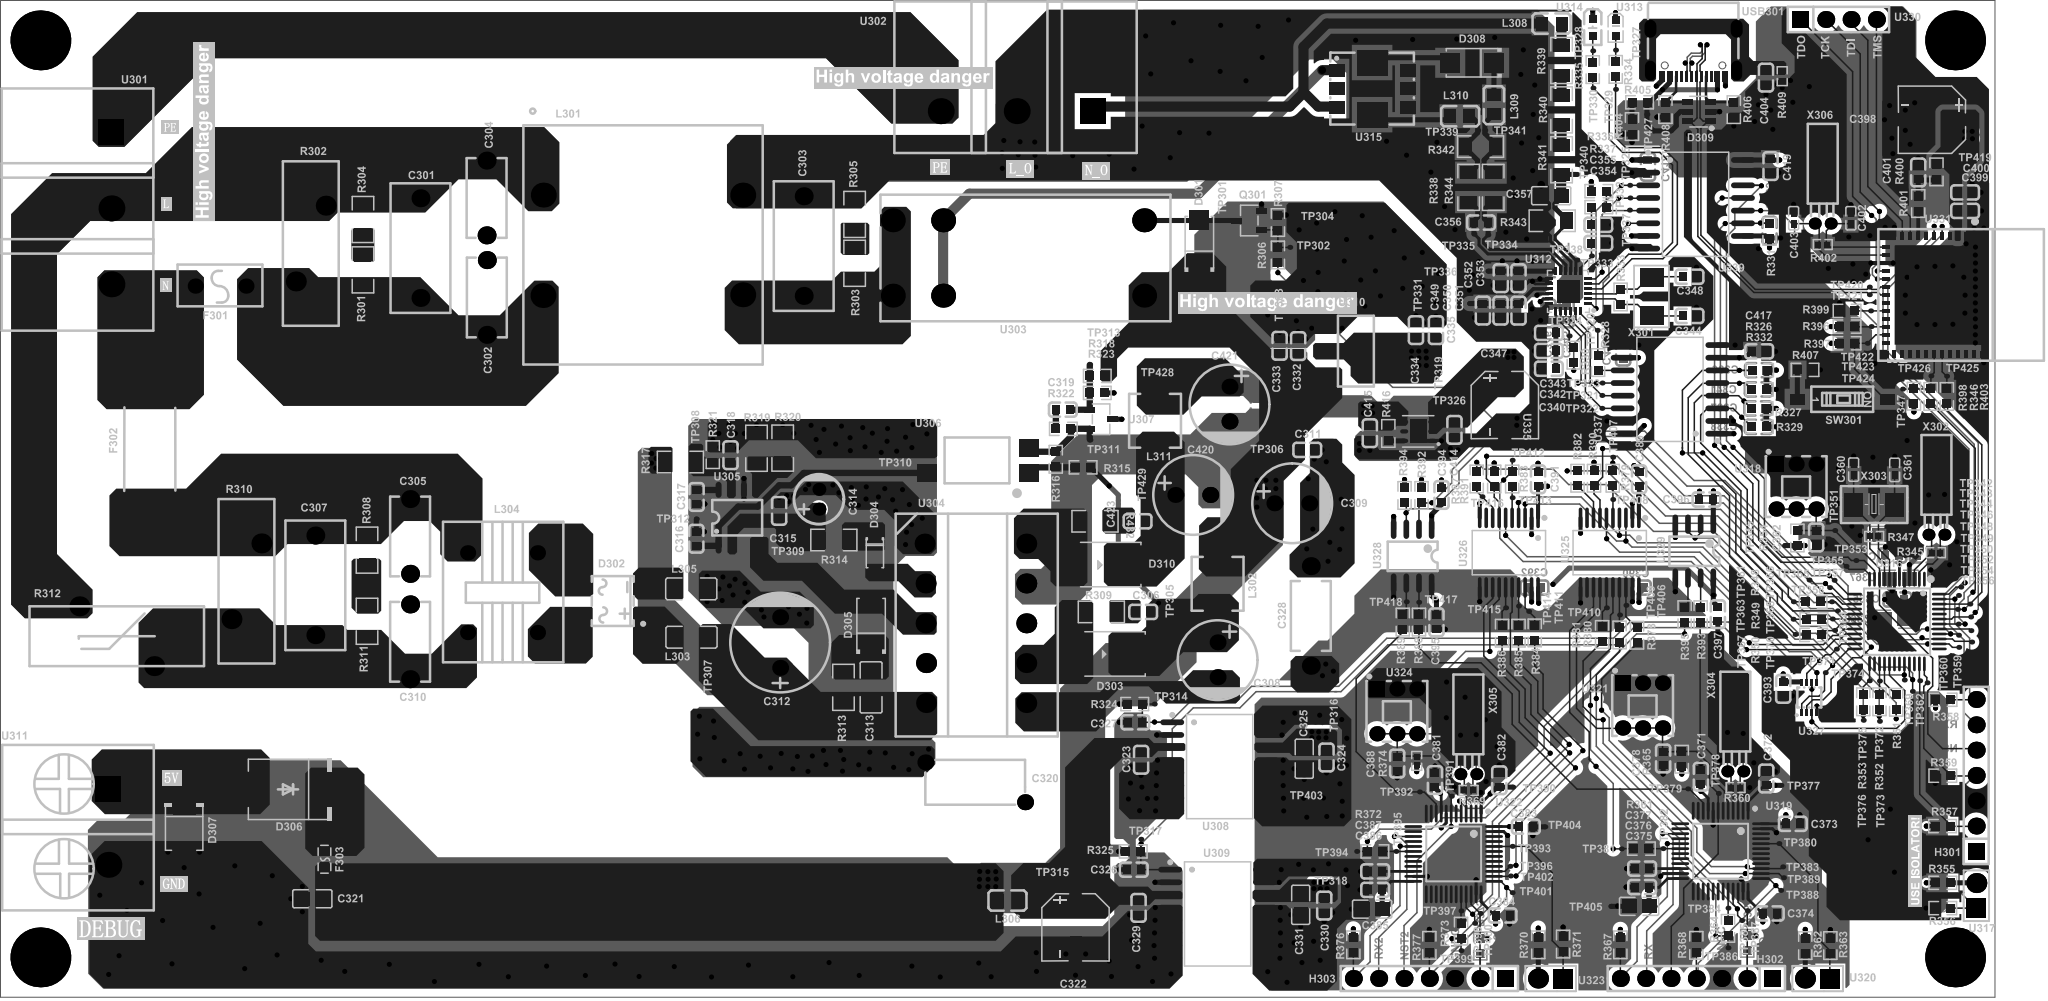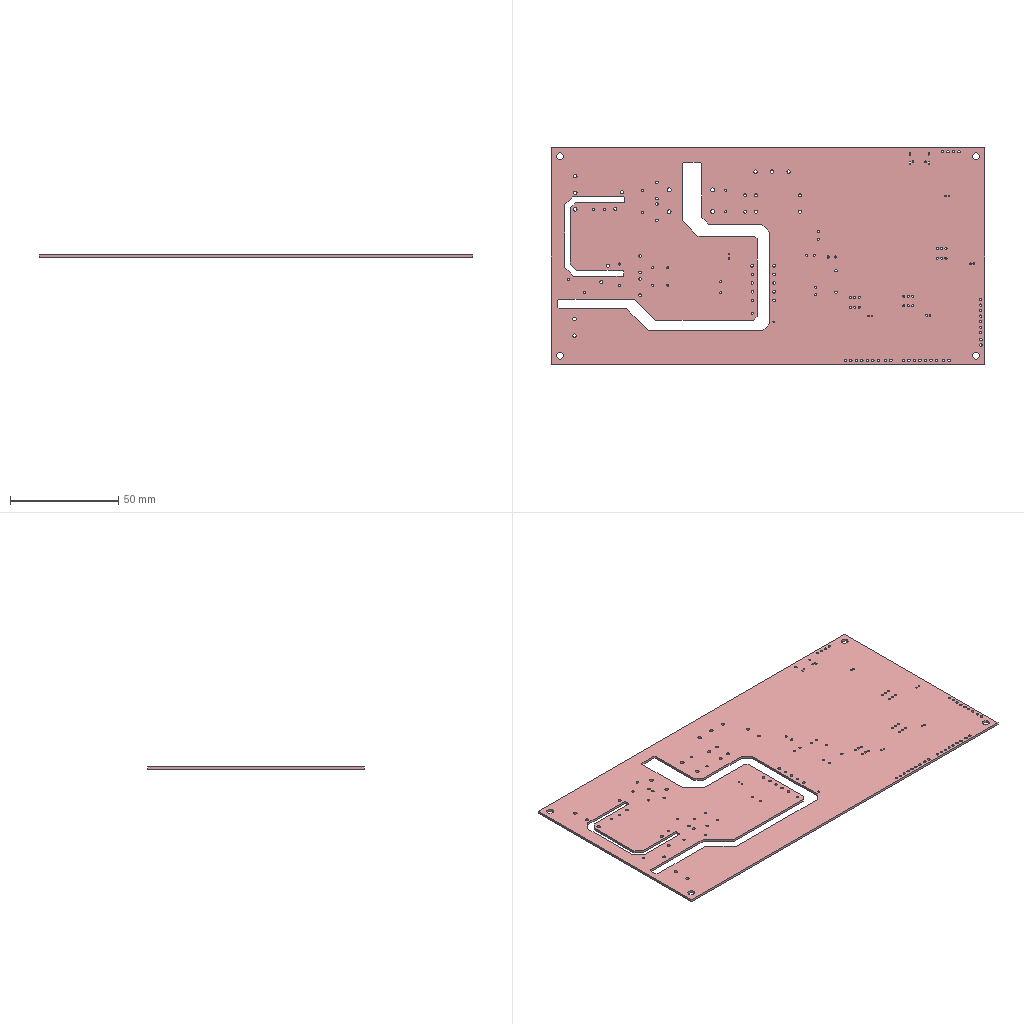Circuit board layout | Altium Designer | box 200 x 100 x 1.1 mm
Layer stack:
# Altium Designer layer stack of  (unit mm; dielectric type: 0 none, 1 core, 2 prepreg, 3 surface material)
index,name,kind,layer,copper_thickness_mm,dielectric_type,dielectric_thickness_mm,dielectric_material,dielectric_constant
0,Top Paste,other,,,,,,
1,Top Overlay,other,,,,,,
2,Top Solder,dielectric,,,3,0.0102,Solder Resist,3.5
3,Top Layer,copper,Top Layer,0.0356,,,,
4,Dielectric1,dielectric,,,1,0.32,FR-4,4.8
5,GND,copper,GND,0.0356,,,,
6,Dielectric2,dielectric,,,2,0.32,FR-4,4.8
7,POWER,copper,POWER,0.0356,,,,
8,Dielectric3,dielectric,,,1,0.32,FR-4,4.8
9,Bottom Layer,copper,Bottom Layer,0.0356,,,,
10,Bottom Solder,dielectric,,,3,0.0102,Solder Resist,3.5
11,Bottom Overlay,other,,,,,,
12,Bottom Paste,other,,,,,,
# drill layer pairs: low layer,high layer
drill_pair,Top Layer,Bottom Layer
Part placement:
Designator,Comment,Layer,Footprint,Center-X(mm),Center-Y(mm),Rotation
C301,100nF,TopLayer,CAP-TH_L13.0-W6.0-P10.00-D0.6,42.113,75.159,270
C302,2.2nF,TopLayer,CAP-TH_L8.0-W4.0-P7.50-D1.2,48.768,70.206,270
C303,100nF,TopLayer,CAP-TH_L13.0-W6.0-P10.00-D0.6,80.543,75.362,270
C304,2.2nF,TopLayer,CAP-TH_L8.0-W4.0-P7.50-D1.2,48.743,80.188,270
C305,2.2nF,TopLayer,CAP-TH_L8.0-W4.0-P7.50-D1.2,41.072,46.228,90
C306,1nF,TopLayer,C0603,114.579,38.659,180
C307,100nF,TopLayer,CAP-TH_L13.0-W6.0-P10.00-D0.6,31.572,41.326,90
C308,680uF,TopLayer,CAP-TH_BD8.0-P3.50-D0.6-FD,122.047,33.858,270
C309,680uF,TopLayer,CAP-TH_BD8.0-P3.50-D0.6-FD,129.489,49.555,360
C310,2.2nF,TopLayer,CAP-TH_L8.0-W4.0-P7.50-D1.2,41.072,35.662,90
C311,1nF,TopLayer,C0603,131.039,54.915,180
C312,33uF,TopLayer,CAP-TH_BD10.0-P5.00-D1.0-FD,78.181,35.585,90
C313,2.2nF,TopLayer,C1206,87.3,31.09,270
C314,47uF,TopLayer,CAP-TH_BD5.0-P2.00-D0.8-FD,82.067,49.962,90
C315,100nF,TopLayer,C0603,78.08,48.793,90
C316,1nF,TopLayer,C0603,69.774,45.999,270
C317,47nF,TopLayer,C0603,69.799,50.19,90
C318,1nF,TopLayer,C0603,73.203,54.381,270
C319,100nF,TopLayer,C0603,106.528,58.953,360
C320,2.2nF,TopLayer,CAP-TH_L10.0-W4.5-P10.00-D0.6-S4.0,97.739,21.565,0
C321,10uF,TopLayer,C0805,31.267,9.881,360
C322,100uF,TopLayer,CAP-SMD_BD6.3-L6.6-W6.6-LS7.2-FD,107.797,7.011,270
C323,22uF,TopLayer,C0603,114.376,23.825,90
C324,100nF,TopLayer,C0603,132.969,24.054,270
C325,10uF,TopLayer,C0805,130.734,23.927,90
C326,1uF,TopLayer,C0603,113.64,12.802,360
C327,1uF,TopLayer,C0603,113.792,27.584,360
C328,100pF,TopLayer,CAP-TH_L7.0-W4.0-P10.00-D0.6,131.394,38.252,270
C329,22uF,TopLayer,C0603,114.122,8.966,90
C330,100nF,TopLayer,C0603,132.74,9.195,270
C331,10uF,TopLayer,C0805,130.378,9.271,90
C332,2.2uF,TopLayer,C0603,130.124,65.329,270
C333,100nF,TopLayer,C0603,128.266,65.359,90
C334,4.7uF,TopLayer,C0603,141.935,66.929,270
C335,100nF,TopLayer,C0603,143.942,66.929,90
C336,150pF,BottomLayer,C0603,176.332,62.912,360
C337,150pF,BottomLayer,C0603,176.256,59.077,360
C338,150pF,BottomLayer,C0603,176.307,57.223,360
C339,150pF,BottomLayer,C0603,177.394,76.911,270
C340,100nF,TopLayer,C0603,155.27,63.057,180
C341,150pF,BottomLayer,C0603,176.307,60.982,360
C342,150pF,TopLayer,C0603,155.27,64.841,180
C343,4.7uF,TopLayer,C0603,155.27,66.65,360
C344,15pF,TopLayer,C0603,169.367,68.351,180
C345,150pF,BottomLayer,C0603,157.048,68.605,270
C346,100nF,BottomLayer,C0603,155.219,68.605,270
C347,100uF,TopLayer,CAP-SMD_BD6.3-L6.6-W6.6-LS7.3-FD-H7.7,150.851,59.411,270
C348,15pF,TopLayer,C0603,169.367,72.288,180
C349,150pF,TopLayer,C0603,148.648,68.891,90
C350,100nF,TopLayer,C0603,150.419,68.885,90
C351,1uF,TopLayer,C0603,152.222,68.885,90
C352,150pF,TopLayer,C0603,150.444,72.136,90
C353,100nF,TopLayer,C0603,152.222,72.136,90
C354,150pF,TopLayer,C0603,160.223,75.667,180
C355,100nF,TopLayer,C0603,160.223,77.495,180
C356,10nF,TopLayer,C0603,148.463,77.724,180
C357,22nF,TopLayer,C0805,155.499,80.416,360
C358,15pF,BottomLayer,C0402,193.345,49.073,270
C359,15pF,BottomLayer,C0402,194.945,49.073,90
C360,30pF,TopLayer,C0402,185.826,52.934,90
C361,30pF,TopLayer,C0402,189.941,52.908,270
C362,1uF,TopLayer,C0603,182.067,46.126,90
C363,100nF,BottomLayer,C0603,189.713,44.323,180
C364,100nF,BottomLayer,C0603,192.862,44.323,360
C365,100nF,BottomLayer,C0603,190.221,39.903,180
C366,10uF,BottomLayer,C0805,189.408,46.33,360
C367,10uF,BottomLayer,C0805,190.424,41.935,360
C368,10uF,BottomLayer,C0805,189.941,37.922,360
C369,15pF,BottomLayer,C0402,173.177,25.121,270
C370,15pF,BottomLayer,C0402,174.752,25.121,90
C371,100nF,TopLayer,C0603,170.51,22.123,90
C372,100nF,TopLayer,C0603,177.063,21.946,90
C373,100nF,TopLayer,C0603,179.73,17.399,360
C374,100nF,TopLayer,C0603,177.419,8.407,360
C375,10uF,TopLayer,C0805,164.313,9.119,360
C376,1nF,TopLayer,C0603,164.617,11.049,360
C377,4.7uF,TopLayer,C0603,164.617,12.903,180
C378,1uF,TopLayer,C0603,166.726,23.952,90
C379,15pF,BottomLayer,C0402,146.406,24.841,270
C380,15pF,BottomLayer,C0402,147.98,24.841,90
C381,100nF,TopLayer,C0603,143.84,21.793,90
C382,100nF,TopLayer,C0603,150.292,21.768,90
C383,100nF,TopLayer,C0603,152.959,17.12,360
C384,100nF,TopLayer,C0603,150.622,8.204,360
C385,10uF,TopLayer,C0805,137.541,8.839,360
C386,1nF,TopLayer,C0603,137.846,10.77,360
C387,4.7uF,TopLayer,C0603,137.846,12.624,180
C388,1uF,TopLayer,C0603,140.056,23.444,90
C389,100nF,TopLayer,C0603,164.313,51.968,90
C390,100nF,BottomLayer,C0603,164.084,41.097,180
C391,100nF,TopLayer,C0603,154.178,51.968,90
C392,100nF,BottomLayer,C0603,153.822,41.097,180
C393,100nF,TopLayer,C0603,178.765,30.937,270
C394,100nF,TopLayer,C0603,144.501,50.394,90
C395,100nF,TopLayer,C0603,143.993,37.617,270
C396,100nF,TopLayer,C0603,171.069,49.936,180
C397,100nF,TopLayer,C0603,172.212,38.43,270
C398,100uF,TopLayer,CAP-SMD_BD6.3-L6.6-W6.6-LS7.2-FD,193.675,88.037,180
C399,100nF,TopLayer,C0603,197.002,78.892,180
C400,22uF,TopLayer,C0603,197.002,80.747,360
C401,1uF,TopLayer,C0603,192.303,82.753,270
C402,15pF,TopLayer,C0402,185.547,78.156,270
C403,15pF,TopLayer,C0402,179.807,78.156,90
C404,10nF,TopLayer,C0603,177.038,92.264,90
D301,SS14,TopLayer,SMA_L4.3-W2.6-LS5.2-RD,120.218,75.743,90
D302,MB10S-50MIL,TopLayer,MBS_L4.7-W3.8-P2.40-LS7.0-TL,61.392,39.751,180
D303,SB10100L,TopLayer,TO-277A_L4.7-W6.1-LS6.6-TR,110.947,34.442,180
D304,BAV21W,TopLayer,SOD-123_L2.8-W1.8-LS3.7-RD,87.681,44.501,270
D305,FR107(RS1M),TopLayer,SMA_L4.3-W2.6-LS5.2-RD,87.3,37.414,90
D306,SS34,TopLayer,SMC_L6.9-W5.9-LS7.9-RD,28.829,20.853,180
D307,SMBJ5.0A,TopLayer,SMB_L4.6-W3.6-LS5.4-RD,18.415,16.967,270
D308,SS14,TopLayer,SMA_L4.3-W2.6-LS5.2-RD,147.574,93.751,180
D309,SRV05-4,TopLayer,SOT-23-6_L2.9-W1.6-P0.95-LS2.8-BL,170.282,88.849,90
F301,20A250VVS,TopLayer,FUSE-TH_L8.4-W4.0-P5.08-D0.6,22.073,71.349,0
F302,SGT520-2A T2AL250V,TopLayer,FUSE-SMD_L20.0-W5.0,14.986,54.966,270
F303,SMD0603-010-15,TopLayer,F0603,32.487,13.843,90
H301,PZ254V-11-07P,TopLayer,HDR-TH_7P-P2.54-V-M,198.119,22.252,90
H302,PZ254V-11-07P,TopLayer,HDR-TH_7P-P2.54-V-M,170.053,1.88,180
H303,PZ254V-11-07P,TopLayer,HDR-TH_7P-P2.54-V-M,143.281,1.88,180
L301,FC-DLFW2015-5mH-20A-LF,TopLayer,FILTER-TH_FC-DLFW2015-5MH-20A-LF,64.414,75.438,270
L302,4.7uH,TopLayer,IND-SMD_L5.4-W5.2_FXL0530,122.047,41.478,90
L303,,TopLayer,L1206,69.291,36.119,0
L304,DLSF1010-12mH-L-S,TopLayer,IND-TH_4P-L14.0-W12.0_DLSF1010-12MH-L-S,50.343,40.589,270
L305,,TopLayer,L1206,69.266,40.97,0
L306,BLM21PG221SN1D,TopLayer,L0805,101.016,9.703,360
L307,,BottomLayer,L0805,156.21,73.254,180
L308,,TopLayer,L0805,155.575,97.688,360
L309,,TopLayer,L0805,149.758,89.535,90
L310,,TopLayer,L0805,146.329,88.392,180
Q301,MMBT3904LT1G,TopLayer,SOT-23-3_L2.9-W1.6-P1.90-LS2.8-BR,125.222,77.927,360
R301,,TopLayer,R1206,36.347,72.974,270
R302,430pF@1kHz,TopLayer,RES-TH_L16.5-W5.6-P7.50-D1.2-S3.00,31.115,75.616,270
R303,,TopLayer,R1206,85.649,73.635,270
R304,,TopLayer,R1206,36.347,78.029,270
R305,,TopLayer,R1206,85.649,78.537,270
R306,,TopLayer,R0603,128.092,74.473,90
R307,,TopLayer,R0603,128.092,77.724,90
R308,,TopLayer,R1206,36.754,44.856,90
R309,,TopLayer,R1206,110.388,38.659,360
R310,430pF@1kHz,TopLayer,RES-TH_L16.5-W5.6-P7.50-D1.2-S3.00,24.663,41.732,90
R311,,TopLayer,R1206,36.754,37.719,90
R312,MF72 20D15,TopLayer,RES-TH_L17.5-W6.0-P7.50-D0.8-S7.50,11.659,36.22,360
R313,,TopLayer,R1206,84.531,31.09,270
R314,,TopLayer,R1206,83.566,45.872,360
R315,,TopLayer,R0603,108.56,53.162,360
R316,,TopLayer,R0603,105.816,53.975,270
R317,,TopLayer,R1206,68.174,53.696,360
R318,,TopLayer,R0603,109.982,62.332,360
R319,,TopLayer,R1206,75.809,55.076,270
R320,,TopLayer,R1206,78.435,55.093,270
R321,,TopLayer,R0603,71.425,54.432,270
R322,,TopLayer,R0603,106.578,57.023,180
R323,,TopLayer,R0603,109.982,60.63,180
R324,,TopLayer,R0603,113.741,29.413,180
R325,,TopLayer,R0603,113.589,14.63,180
R326,,TopLayer,R0603,176.394,62.918,180
R327,,TopLayer,R0603,176.344,59.074,180
R328,,TopLayer,R0603,160.198,63.678,270
R329,,TopLayer,R0603,176.369,57.229,180
R330,,TopLayer,R0603,157.759,64.414,270
R331,,TopLayer,R0603,177.391,76.849,90
R332,,TopLayer,R0603,176.369,60.985,180
R333,,TopLayer,R0603,162.458,70.256,270
R334,,TopLayer,R0603,161.969,93.09,270
R335,,TopLayer,R0603,159.664,93.066,270
R336,,TopLayer,R0603,160.274,80.874,180
R337,,TopLayer,R0603,160.274,79.273,360
R338,,TopLayer,R1206,147.218,81.255,90
R339,,TopLayer,R1206,156.54,93.98,90
R340,,TopLayer,R1206,156.54,89.027,270
R341,,TopLayer,R1206,156.54,84.023,90
R342,,TopLayer,R1206,148.412,85.344,180
R343,,TopLayer,R1206,155.6,77.902,360
R344,,TopLayer,R1206,149.685,81.249,90
R345,,TopLayer,R0402,194.081,44.602,180
R346,,TopLayer,R0603,193.548,60.274,270
R347,,TopLayer,R0402,187.884,46.228,180
R348,,TopLayer,R0603,181.762,39.675,180
R349,,TopLayer,R0603,181.839,37.922,180
R350,,TopLayer,R0603,181.813,36.347,180
R351,,TopLayer,R0603,190.094,29.591,90
R352,,TopLayer,R0603,188.417,29.642,90
R353,,TopLayer,R0603,186.792,29.642,90
R354,,TopLayer,R0603,180.188,46.076,270
R355,,TopLayer,R0603,194.767,11.481,180
R356,,TopLayer,R0603,194.767,8.941,180
R357,,TopLayer,R0603,194.742,17.17,180
R358,,TopLayer,R0603,194.793,29.845,180
R359,,TopLayer,R0603,194.767,22.225,180
R360,,TopLayer,R0402,173.99,21.031,180
R361,,TopLayer,R0603,164.541,14.91,180
R362,,TopLayer,R0603,180.975,5.182,90
R363,,TopLayer,R0603,183.49,5.182,90
R364,,TopLayer,R0603,173.228,6.909,90
R365,,TopLayer,R0603,168.594,23.879,270
R366,,BottomLayer,R0603,175.158,5.41,90
R367,,TopLayer,R0603,162.433,5.258,90
R368,,TopLayer,R0603,170.053,5.207,90
R369,,TopLayer,R0402,147.218,20.752,180
R370,,TopLayer,R0603,154.203,5.258,90
R371,,TopLayer,R0603,156.693,5.334,270
R372,,TopLayer,R0603,137.82,14.63,180
R373,,TopLayer,R0603,146.456,6.629,90
R374,,TopLayer,R0402,142.01,23.71,270
R375,,BottomLayer,R0603,148.387,5.131,90
R376,,TopLayer,R0603,135.661,5.258,90
R377,,TopLayer,R0603,143.281,5.207,90
R378,,TopLayer,R0603,164.109,36.322,90
R379,,TopLayer,R0603,161.671,52.07,90
R380,,TopLayer,R0603,162.357,36.347,90
R381,,TopLayer,R0603,160.604,36.398,90
R382,,TopLayer,R0603,158.14,52.07,90
R383,,TopLayer,R0603,151.587,51.994,90
R384,,TopLayer,R0603,153.848,36.551,90
R385,,TopLayer,R0603,152.222,36.525,90
R386,,TopLayer,R0603,150.571,36.525,90
R387,,TopLayer,R0603,148.031,51.994,90
R388,,TopLayer,R0603,142.24,37.643,90
R389,,TopLayer,R0603,140.614,37.643,90
R390,,TopLayer,R0603,159.791,52.07,270
R391,,TopLayer,R0603,149.784,51.994,270
R392,,TopLayer,R0603,142.494,50.343,90
R393,,TopLayer,R0603,170.485,38.379,90
R394,,TopLayer,R0603,140.792,50.343,90
R395,,TopLayer,R0603,168.878,38.382,90
R396,,TopLayer,R0603,185.166,67.285,180
R397,,TopLayer,R0603,185.166,65.608,180
R398,,TopLayer,R0603,191.872,60.3,270
R399,,TopLayer,R0603,185.166,68.859,360
R400,,TopLayer,R0603,194.132,82.804,90
R401,,TopLayer,R0603,192.303,79.629,270
R402,,TopLayer,R0402,182.728,75.514,360
R403,,TopLayer,R0603,195.174,60.274,90
R404,,TopLayer,R0603,163.601,87.351,270
R405,,TopLayer,R0603,164.363,89.789,360
R406,,TopLayer,R0603,173.812,89.052,90
R407,,TopLayer,R0603,180.95,62.941,180
R408,,TopLayer,R0603,166.954,89.052,90
R409,,TopLayer,R0402,178.664,92.405,90
SW301,U903,TopLayer,SW-SMD_2P-L3.5-W6.1-P2.54-LS9.8,184.683,59.995,360
TP301,,TopLayer,Test-Point-0.5mm,122.326,77.927,180
TP302,,TopLayer,Test-Point-0.5mm,129.286,75.235,90
TP303,,TopLayer,Test-Point-0.5mm,128.27,67.335,90
TP304,,TopLayer,Test-Point-0.5mm,129.642,78.486,90
TP305,,TopLayer,Test-Point-0.5mm,117.069,37.694,0
TP306,,TopLayer,Test-Point-0.5mm,128.905,54.889,180
TP307,,TopLayer,Test-Point-0.5mm,70.866,34.29,0
TP308,,TopLayer,Test-Point-0.5mm,69.647,55.194,0
TP309,,TopLayer,Test-Point-0.5mm,78.08,46.736,0
TP310,,TopLayer,Test-Point-0.5mm,90.703,52.603,0
TP311,,TopLayer,Test-Point-0.5mm,109.245,55.905,0
TP312,,TopLayer,Test-Point-0.5mm,69.774,47.981,0
TP313,,TopLayer,Test-Point-0.5mm,109.22,63.475,0
TP314,,TopLayer,Test-Point-0.5mm,115.697,29.413,360
TP315,,TopLayer,Test-Point-0.5mm,107.772,12.395,180
TP316,,TopLayer,Test-Point-0.5mm,133.604,26.086,360
TP317,,TopLayer,Test-Point-0.5mm,114.351,15.85,360
TP318,,TopLayer,Test-Point-0.5mm,133.68,10.973,360
TP319,,TopLayer,Test-Point-0.5mm,143.815,64.643,360
TP320,,TopLayer,Test-Point-0.5mm,160.122,66.904,180
TP321,,TopLayer,Test-Point-0.5mm,160.579,60.376,270
TP322,,TopLayer,Test-Point-0.5mm,160.579,59.08,270
TP323,,TopLayer,Test-Point-0.5mm,160.604,61.62,270
TP324,,TopLayer,Test-Point-0.5mm,157.302,66.345,180
TP325,,TopLayer,Test-Point-0.5mm,163.373,81.458,360
TP326,,TopLayer,Test-Point-0.5mm,145.796,59.055,180
TP327,,TopLayer,Test-Point-0.5mm,161.95,95.021,180
TP328,,TopLayer,Test-Point-0.5mm,159.664,94.945,180
TP329,,TopLayer,Test-Point-0.5mm,161.95,91.084,180
TP330,,TopLayer,Test-Point-0.5mm,159.69,91.211,180
TP331,,TopLayer,Test-Point-0.5mm,147.32,69.596,90
TP332,,TopLayer,Test-Point-0.5mm,163.398,80.188,360
TP333,,TopLayer,Test-Point-0.5mm,158.09,73.965,90
TP334,,TopLayer,Test-Point-0.5mm,149.149,76.479,90
TP335,,TopLayer,Test-Point-0.5mm,147.752,76.556,90
TP336,,TopLayer,Test-Point-0.5mm,149.174,72.847,90
TP337,,TopLayer,Test-Point-0.5mm,163.347,78.969,90
TP338,,TopLayer,Test-Point-0.5mm,159.537,74.371,90
TP339,,TopLayer,Test-Point-0.5mm,148.133,86.97,90
TP340,,TopLayer,Test-Point-0.5mm,158.064,82.55,90
TP341,,TopLayer,Test-Point-0.5mm,148.844,86.97,90
TP342,,TopLayer,Test-Point-0.5mm,196.571,41.148,360
TP343,,TopLayer,Test-Point-0.5mm,196.342,40.31,360
TP344,,TopLayer,Test-Point-0.5mm,197.485,39.446,360
TP345,,TopLayer,Test-Point-0.5mm,178.918,45.314,180
TP346,,TopLayer,Test-Point-0.5mm,196.24,38.913,360
TP347,,TopLayer,Test-Point-0.5mm,190.729,61.011,270
TP348,,TopLayer,Test-Point-0.5mm,197.561,38.151,360
TP349,,TopLayer,Test-Point-0.5mm,196.317,37.44,360
TP350,,TopLayer,Test-Point-0.5mm,197.587,36.779,360
TP351,,TopLayer,Test-Point-0.5mm,183.933,46.826,180
TP352,,TopLayer,Test-Point-0.5mm,196.342,36.322,360
TP353,,TopLayer,Test-Point-0.5mm,186.055,43.815,180
TP354,,TopLayer,Test-Point-0.5mm,197.663,35.636,360
TP355,,TopLayer,Test-Point-0.5mm,185.064,43.231,180
TP356,,TopLayer,Test-Point-0.5mm,196.367,35.103,360
TP357,,TopLayer,Test-Point-0.5mm,183.871,41.834,180
TP358,,TopLayer,Test-Point-0.5mm,183.413,41.097,180
TP359,,TopLayer,Test-Point-0.5mm,193.192,31.547,360
TP360,,TopLayer,Test-Point-0.5mm,192.456,31.75,360
TP361,,TopLayer,Test-Point-0.5mm,179.781,39.675,180
TP362,,TopLayer,Test-Point-0.5mm,191.719,30.683,270
TP363,,TopLayer,Test-Point-0.5mm,179.756,37.922,180
TP364,,TopLayer,Test-Point-0.5mm,184.201,38.76,180
TP365,,TopLayer,Test-Point-0.5mm,181.356,41.859,180
TP366,,TopLayer,Test-Point-0.5mm,183.617,39.675,180
TP367,,TopLayer,Test-Point-0.5mm,179.959,36.398,180
TP368,,TopLayer,Test-Point-0.5mm,183.693,37.948,180
TP369,,TopLayer,Test-Point-0.5mm,190.906,31.826,270
TP370,,TopLayer,Test-Point-0.5mm,183.921,36.805,180
TP371,,TopLayer,Test-Point-0.5mm,184.099,34.925,180
TP372,,TopLayer,Test-Point-0.5mm,188.417,31.725,270
TP373,,TopLayer,Test-Point-0.5mm,188.417,27.686,180
TP374,,TopLayer,Test-Point-0.5mm,182.982,32.563,180
TP375,,TopLayer,Test-Point-0.5mm,187.401,31.75,270
TP376,,TopLayer,Test-Point-0.5mm,186.792,27.788,180
TP377,,TopLayer,Test-Point-0.5mm,178.537,21.26,180
TP378,,TopLayer,Test-Point-0.5mm,172.263,20.447,180
TP379,,TopLayer,Test-Point-0.5mm,169.189,20.904,180
TP380,,TopLayer,Test-Point-0.5mm,178.333,15.418,180
TP381,,TopLayer,Test-Point-0.5mm,162.535,14.884,180
TP382,,TopLayer,Test-Point-0.5mm,166.7,14.91,180
TP383,,TopLayer,Test-Point-0.5mm,178.714,13.081,180
TP384,,TopLayer,Test-Point-0.5mm,173.228,8.941,180
TP385,,TopLayer,Test-Point-0.5mm,174.6,7.696,180
TP386,,TopLayer,Test-Point-0.5mm,173.228,4.953,180
TP387,,TopLayer,Test-Point-0.5mm,175.158,8.687,180
TP388,,TopLayer,Test-Point-0.5mm,178.511,10.719,180
TP389,,TopLayer,Test-Point-0.5mm,178.791,11.989,180
TP390,,TopLayer,Test-Point-0.5mm,151.638,21.082,180
TP391,,TopLayer,Test-Point-0.5mm,145.491,20.168,180
TP392,,TopLayer,Test-Point-0.5mm,142.291,20.599,180
TP393,,TopLayer,Test-Point-0.5mm,151.587,15.138,180
TP394,,TopLayer,Test-Point-0.5mm,135.992,14.63,180
TP395,,TopLayer,Test-Point-0.5mm,139.929,14.63,180
TP396,,TopLayer,Test-Point-0.5mm,151.359,13.132,180
TP397,,TopLayer,Test-Point-0.5mm,146.456,8.661,180
TP398,,TopLayer,Test-Point-0.5mm,147.828,7.417,180
TP399,,TopLayer,Test-Point-0.5mm,146.456,4.674,180
TP400,,TopLayer,Test-Point-0.5mm,148.387,8.407,180
TP401,,TopLayer,Test-Point-0.5mm,151.587,10.49,180
TP402,,TopLayer,Test-Point-0.5mm,151.409,12.167,180
TP403,,TopLayer,Test-Point-0.5mm,130.734,21.285,180
TP404,,TopLayer,Test-Point-0.5mm,154.864,17.094,180
TP405,,TopLayer,Test-Point-0.5mm,161.493,9.119,180
TP406,,TopLayer,Test-Point-0.5mm,162.992,39.319,270
TP407,,TopLayer,Test-Point-0.5mm,161.671,54.178,270
TP408,,TopLayer,Test-Point-0.5mm,161.671,49.936,270
TP409,,TopLayer,Test-Point-0.5mm,162.357,38.354,270
TP410,,TopLayer,Test-Point-0.5mm,161.036,39.065,270
TP411,,TopLayer,Test-Point-0.5mm,153.238,38.71,270
TP412,,TopLayer,Test-Point-0.5mm,151.587,53.873,270
TP413,,TopLayer,Test-Point-0.5mm,151.587,50.114,270
TP414,,TopLayer,Test-Point-0.5mm,152.222,39.243,270
TP415,,TopLayer,Test-Point-0.5mm,150.927,39.065,270
TP416,,TopLayer,Test-Point-0.5mm,148.564,50.216,270
TP417,,TopLayer,Test-Point-0.5mm,142.215,39.624,270
TP418,,TopLayer,Test-Point-0.5mm,140.97,39.675,270
TP419,,TopLayer,Test-Point-0.5mm,196.291,82.499,270
TP420,,TopLayer,Test-Point-0.5mm,187.401,71.247,270
TP421,,TopLayer,Test-Point-0.5mm,187.401,70.485,270
TP422,,TopLayer,Test-Point-0.5mm,187.528,68.859,270
TP423,,TopLayer,Test-Point-0.5mm,187.579,67.285,270
TP424,,TopLayer,Test-Point-0.5mm,187.198,65.608,270
TP425,,TopLayer,Test-Point-0.5mm,195.148,62.306,270
TP426,,TopLayer,Test-Point-0.5mm,193.573,62.332,270
TP427,,TopLayer,Test-Point-0.5mm,165.1,88.57,180
U301,DBT50G-7.62-3P-BK-P,TopLayer,CONN-TH_3P-P7.62_L15.2-W24.4-EX4.2,11.125,79.146,270
U302,DBT50G-7.62-3P-BK-P,TopLayer,CONN-TH_3P-P7.62_L15.2-W24.4-EX4.2,101.905,88.9,180
U303,HF115F-I/005-1HS3A,TopLayer,RELAY-TH_HF115F-XXX-1HS3,102.083,74.168,180
U304,,TopLayer,111,97.763,37.514,0
U305,HF500GS-15-Z,TopLayer,SOIC-8_7P-L4.9-W3.9-P1.27-LS6.0-BL-PE3,73.914,48.108,0
U306,PC817AS,TopLayer,SOP-4_L6.5-W4.6-P2.54-LS10.2-TL,97.993,53.873,180
U307,TL431KB-TP,TopLayer,SOT-23-3_L2.9-W1.4-P1.91-LS2.6-BR,110.363,57.988,180
U308,CA-IS3115AW,TopLayer,SOIC-16_L10.3-W7.5-P1.27-LS10.3-BL,122.25,23.139,270
U309,CA-IS3115AW,TopLayer,SOIC-16_L10.3-W7.5-P1.27-LS10.3-BL,122.047,8.357,270
U310,TLV1117LV33DCYR,TopLayer,SOT-223_L6.7-W3.5-P2.30-BR,135.915,64.821,180
U311,DBT50G-7.62-2P-BK-P,TopLayer,CONN-TH_2P-P7.62_L15.2-W16.7-EX4.2,10.82,17.094,270
U312,STPM32TR,TopLayer,VQFN-24_L4.0-W4.0-P0.50-BL-EP2.3,157.226,70.815,90
U313,19-217/GHC-YR1S2/6T,TopLayer,LED0603-RD_GREEN,161.951,97.206,270
U314,19-217/R6C-AL1M2VY/6T,TopLayer,LED0603-R-FD,159.664,97.307,270
U315,PA1005.100NL,TopLayer,SENSOR-TH_PA1005.100NL,137.541,91.161,90
U316,STM32G071CBT6,TopLayer,LQFP-48_L7.0-W7.0-P0.50-LS9.0-BL,190.17,37.694,180
U317,PZ254V-11-02P,TopLayer,HDR-TH_2P-P2.54-V-M,198.133,10.185,90
U318,5.8 ZSGT,TopLayer,SW-TH_5.8ZSGT,180.061,51.232,180
U319,STM32U575CGT6,TopLayer,LQFP-48_L7.0-W7.0-P0.50-LS9.0-TL,172.491,14.656,270
U320,PZ254V-11-02P,TopLayer,HDR-TH_2P-P2.54-V-M,182.219,1.874,180
U321,5.8 ZSGT,TopLayer,SW-TH_5.8ZSGT,164.664,29.264,180
U322,STM32U575CGT6,TopLayer,LQFP-48_L7.0-W7.0-P0.50-LS9.0-TL,145.72,14.376,270
U323,PZ254V-11-02P,TopLayer,HDR-TH_2P-P2.54-V-M,155.448,1.874,180
U324,5.8 ZSGT,TopLayer,SW-TH_5.8ZSGT,140.026,28.68,180
U325,ADUM3150BRSZ-RL7,TopLayer,SSOP-20_L7.2-W5.3-P0.65-LS7.8-BL,161.366,44.602,180
U326,ADUM3150BRSZ-RL7,TopLayer,SSOP-20_L7.2-W5.3-P0.65-LS7.8-BL,151.257,44.602,180
U327,SN74LVC2G125DCUR,TopLayer,VSON8_L2.0-W2.3-P0.50-LS3.1-BL,181.381,30.074,360
U328,ISO7720FDR,TopLayer,SOIC-8_L5.0-W4.0-P1.27-LS6.1-BL,141.605,44.247,180
U329,ISO7720FDR,TopLayer,SOIC-8_L5.0-W4.0-P1.27-LS6.1-BL,169.85,44.755,180
U330,PZ254V-11-04P,TopLayer,HDR-TH_4P-P2.54-V-M,184.302,98.095,360
U331,ESP32-C6-MINI-1-N4,TopLayer,WIFIM-SMD_61P-L16.6-W13.2-P0.80-ESP32-C6-MINI-1-N4,193.929,70.46,270
USB301,TYPE-C 16PIN 2MD(073),TopLayer,USB-C-SMD_TYPE-C-6PIN-2MD-073,169.774,94.793,180
X301,16MHz,TopLayer,CRYSTAL-SMD_2P-L5.0-W3.2,165.557,70.307,270
U335,LDL212PU33R,TopLayer,VSON-6_L3.0-W3.0-P0.95-TL-EP_TI_DRP,142.164,56.769,180
R416,,TopLayer,R0603,139.167,56.566,270
X304,32.768kHz,TopLayer,OSC-TH_BD3.1-P0.8-D0.3,173.965,22.657,270
X305,32.768kHz,TopLayer,OSC-TH_BD3.1-P0.8-D0.3,147.193,22.377,270
X306,32.768kHz,TopLayer,OSC-TH_BD3.1-P0.8-D0.3,182.728,77.622,270
C414,4.7uF,TopLayer,C0603,145.796,56.921,90
C415,1uF,TopLayer,C0603,137.312,56.591,90
C416,100nF,BottomLayer,C0603,162.712,64.77,90
C417,100nF,TopLayer,C0603,176.352,64.795,360
C418,100nF,BottomLayer,C0603,165.202,83.312,270
C419,100nF,TopLayer,C0603,177.495,83.388,270
C420,680uF,TopLayer,CAP-TH_BD8.0-P3.50-D0.6-FD,119.558,50.394,360
C421,680uF,TopLayer,CAP-TH_BD8.0-P3.50-D0.6-FD,123.241,59.512,270
C422,1nF,BottomLayer,C0603,126.086,59.36,90
C423,1nF,TopLayer,C0603,114.021,47.752,180
D310,SB10100L,TopLayer,TO-277A_L4.7-W6.1-LS6.6-TR,110.515,43.409,180
L311,4.7uH,TopLayer,IND-SMD_L5.4-W5.2_FXL0530,115.773,57.836,90
R432,,TopLayer,R1206,109.753,47.752,360
TP428,,TopLayer,Test-Point-0.5mm,115.799,61.671,90
TP429,,TopLayer,Test-Point-0.5mm,114.376,53.645,90
U337,ISO7741FDWR,TopLayer,SOIC-16_L10.3-W7.5-P1.27-LS10.3-BL,167.411,60.985,90
U339,ISO7742DWR,TopLayer,SOIC-16_L10.3-W7.5-P1.27-LS10.3-BL,169.977,79.553,270
X302,32.768kHz,TopLayer,OSC-TH_BD3.1-P0.8-D0.3,194.132,46.406,270
X303,8MHz,TopLayer,CRYSTAL-SMD_L5.0-W3.2,187.884,49.428,180
Pad and via stacks, first 67 of 92 lines:
# Altium Designer via and pad stacks of  (unit mm). Each distinct definition once, with the count of objects using it.
# via: kind,start_layer,end_layer,hole_mm,diameter_mm,mode(0 simple;1 top-mid-bottom;2 full stack),diameter_per_layer,count,example_net
# pad: kind,layer,hole_mm,hole_type(0 round;1 square;2 slot),plating,top_size,top_shape(1 round;2 rect;3 octagon;9 rounded rect),mid_size,bottom_size,mode,footprint,size_per_layer,count,example
pad,Multi-Layer,1,0,plated,1.8x1.8,1,1.8x1.8,1.8x1.8,0,CAP-TH_L13.0-W6.0-P10.00-D0.6,,6,C301.2
pad,Multi-Layer,1.2,0,plated,1.8x1.8,1,1.8x1.8,1.8x1.8,0,CAP-TH_L8.0-W4.0-P7.50-D1.2,,8,C302.2
pad,Multi-Layer,1,0,plated,1.6x1.6,1,1.6x1.6,1.6x1.6,0,CAP-TH_BD8.0-P3.50-D0.6-FD,,8,C308.1
pad,Multi-Layer,1,0,plated,1.6x1.6,1,1.6x1.6,1.6x1.6,0,CAP-TH_BD10.0-P5.00-D1.0-FD,,2,C312.2
pad,Multi-Layer,0.8,0,plated,1.3x1.3,1,1.3x1.3,1.3x1.3,0,CAP-TH_BD5.0-P2.00-D0.8-FD,,2,C314.2
pad,Multi-Layer,0.9,0,plated,1.6x1.6,1,1.6x1.6,1.6x1.6,0,CAP-TH_L10.0-W4.5-P10.00-D0.6-S4.0,,2,C320.2
pad,Multi-Layer,1.1,0,plated,1.8x1.8,1,1.8x1.8,1.8x1.8,0,CAP-TH_L7.0-W4.0-P10.00-D0.6,,2,C328.2
pad,Multi-Layer,1,0,plated,1.524x1.524,1,1.524x1.524,1.524x1.524,0,FUSE-TH_L8.4-W4.0-P5.08-D0.6,,2,F301.2
pad,Multi-Layer,1.1,0,plated,1.7x1.7,1,1.7x1.7,1.7x1.7,0,HDR-TH_7P-P2.54-V-M,,18,H301.7
pad,Multi-Layer,1.1,0,plated,1.7x1.7,2,1.7x1.7,1.7x1.7,0,HDR-TH_7P-P2.54-V-M,,3,H301.1
pad,Multi-Layer,1.8,0,plated,2.5x2.5,1,2.5x2.5,2.5x2.5,0,FILTER-TH_FC-DLFW2015-5MH-20A-LF,,4,L301.1
pad,Multi-Layer,1,0,plated,1.524x1.524,1,1.524x1.524,1.524x1.524,0,IND-TH_4P-L14.0-W12.0_DLSF1010-12MH-L-S,,4,L304.4
pad,Multi-Layer,1.4,0,plated,2x2,1,2x2,2x2,0,RES-TH_L16.5-W5.6-P7.50-D1.2-S3.00,,4,R302.2
pad,Multi-Layer,1.2,0,plated,2x2,1,2x2,2x2,0,RES-TH_L17.5-W6.0-P7.50-D0.8-S7.50,,2,R312.2
pad,Multi-Layer,1.6,0,plated,2.6x2.6,1,2.6x2.6,2.6x2.6,0,CONN-TH_3P-P7.62_L15.2-W24.4-EX4.2,,4,U301.3
pad,Multi-Layer,1.6,0,plated,2.6x2.6,2,2.6x2.6,2.6x2.6,0,CONN-TH_3P-P7.62_L15.2-W24.4-EX4.2,,2,U301.1
pad,Multi-Layer,1.4,0,plated,2.4x2.4,1,2.4x2.4,2.4x2.4,0,RELAY-TH_HF115F-XXX-1HS3,,6,U303.2
pad,Multi-Layer,1.2,0,plated,2x2,1,2x2,2x2,0,111,,10,U304.6
pad,Multi-Layer,1.6,0,plated,2.6x2.6,1,2.6x2.6,2.6x2.6,0,CONN-TH_2P-P7.62_L15.2-W16.7-EX4.2,,1,U311.2
pad,Multi-Layer,1.6,0,plated,2.6x2.6,2,2.6x2.6,2.6x2.6,0,CONN-TH_2P-P7.62_L15.2-W16.7-EX4.2,,1,U311.1
pad,Multi-Layer,1.2,0,plated,2x2,1,2x2,2x2,0,HDR-TH_2P-P2.54-V-M,,3,U317.2
pad,Multi-Layer,1.2,0,plated,2x2,2,2x2,2x2,0,HDR-TH_2P-P2.54-V-M,,3,U317.1
pad,Multi-Layer,1,0,plated,1.524x1.524,2,1.524x1.524,1.524x1.524,0,SW-TH_5.8ZSGT,,3,U318.1
pad,Multi-Layer,1,0,plated,1.524x1.524,1,1.524x1.524,1.524x1.524,0,SW-TH_5.8ZSGT,,15,U318.2
pad,Multi-Layer,1.1,0,plated,1.7x1.7,1,1.7x1.7,1.7x1.7,0,HDR-TH_4P-P2.54-V-M,,3,U330.4
pad,Multi-Layer,1.1,0,plated,1.7x1.7,2,1.7x1.7,1.7x1.7,0,HDR-TH_4P-P2.54-V-M,,1,U330.1
pad,Multi-Layer,0.6,2,plated,1.2x1.8,1,1.2x1.8,1.2x1.8,0,USB-C-SMD_TYPE-C-6PIN-2MD-073,,2,USB301.14
pad,Multi-Layer,0.6,2,plated,1.1x2,1,1.1x2,1.1x2,0,USB-C-SMD_TYPE-C-6PIN-2MD-073,,2,USB301.14
pad,Multi-Layer,0.8,0,plated,1.2x1.2,1,1.2x1.2,1.2x1.2,0,OSC-TH_BD3.1-P0.8-D0.3,,8,X306.2
pad,Multi-Layer,3.2,0,plated,6x6,1,6x6,6x6,0,,,4,0
pad,Top Layer,0,0,plated,0.8x0.9,2,0.8x0.9,0.8x0.9,0,C0603,,122,C394.1
pad,Top Layer,0,0,plated,1.485x1.728,2,1.485x1.728,1.485x1.728,0,C1206,,2,C313.1
pad,Top Layer,0,0,plated,1.41x1.35,2,1.41x1.35,1.41x1.35,0,C0805,,12,C321.1
pad,Top Layer,0,0,plated,3.5x1.2,2,3.5x1.2,3.5x1.2,0,CAP-SMD_BD6.3-L6.6-W6.6-LS7.2-FD,,4,C322.1
pad,Top Layer,0,0,plated,3.5x1.2,2,3.5x1.2,3.5x1.2,0,CAP-SMD_BD6.3-L6.6-W6.6-LS7.3-FD-H7.7,,2,C347.2
pad,Top Layer,0,0,plated,0.7901x0.54,2,0.7901x0.54,0.7901x0.54,0,C0402,,8,C360.1
pad,Top Layer,0,0,plated,2x2,2,2x2,2x2,0,SMA_L4.3-W2.6-LS5.2-RD,,6,D301.1
pad,Top Layer,0,0,plated,2x1.1,2,2x1.1,2x1.1,0,MBS_L4.7-W3.8-P2.40-LS7.0-TL,,4,D302.3
pad,Top Layer,0,0,plated,4x3.6,2,4x3.6,4x3.6,0,TO-277A_L4.7-W6.1-LS6.6-TR,,2,D303.3
pad,Top Layer,0,0,plated,1x1.5,2,1x1.5,1x1.5,0,TO-277A_L4.7-W6.1-LS6.6-TR,,4,D303.2
pad,Top Layer,0,0,plated,0.95x1.15,2,0.95x1.15,0.95x1.15,0,SOD-123_L2.8-W1.8-LS3.7-RD,,2,D304.1
pad,Top Layer,0,0,plated,2.7x3.3,2,2.7x3.3,2.7x3.3,0,SMC_L6.9-W5.9-LS7.9-RD,,2,D306.1
pad,Top Layer,0,0,plated,2.047x2.241,2,2.047x2.241,2.047x2.241,0,SMB_L4.6-W3.6-LS5.4-RD,,2,D307.2
pad,Top Layer,0,0,plated,0.532x1.072,2,0.532x1.072,0.532x1.072,0,SOT-23-6_L2.9-W1.6-P0.95-LS2.8-BL,,6,D309.6
pad,Top Layer,0,0,plated,6x6,2,6x6,6x6,0,FUSE-SMD_L20.0-W5.0,,2,F302.2
pad,Top Layer,0,0,plated,0.8065x0.864,2,0.8065x0.864,0.8065x0.864,0,F0603,,2,F303.1
pad,Top Layer,0,0,plated,1.9x2.5,2,1.9x2.5,1.9x2.5,0,IND-SMD_L5.4-W5.2_FXL0530,,4,L302.2
pad,Top Layer,0,0,plated,1.485x1.728,2,1.485x1.728,1.485x1.728,0,L1206,,4,L303.1
pad,Top Layer,0,0,plated,1.133x1.377,2,1.133x1.377,1.133x1.377,0,L0805,,8,L306.2
pad,Top Layer,0,0,plated,1.07x0.6,2,1.07x0.6,1.07x0.6,0,SOT-23-3_L2.9-W1.6-P1.90-LS2.8-BR,,3,Q301.3
pad,Top Layer,0,0,plated,1.208x1.701,2,1.208x1.701,1.208x1.701,0,R1206,,40,R301.1
pad,Top Layer,0,0,plated,0.8065x0.864,2,0.8065x0.864,0.8065x0.864,0,R0603,,158,R306.1
pad,Top Layer,0,0,plated,0.5657x0.54,2,0.5657x0.54,0.5657x0.54,0,R0402,,14,R345.1
pad,Top Layer,0,0,plated,1.1x1.5,2,1.1x1.5,1.1x1.5,0,SW-SMD_2P-L3.5-W6.1-P2.54-LS9.8,,2,SW301.2
pad,Top Layer,0,0,plated,0.5x0.5,1,0.5x0.5,0.5x0.5,0,Test-Point-0.5mm,,129,TP301.1
pad,Top Layer,0,0,plated,0.6x1.6,1,0.6x1.6,0.6x1.6,0,SOIC-8_7P-L4.9-W3.9-P1.27-LS6.0-BL-PE3,,7,U305.1
pad,Top Layer,0,0,plated,1.8x2,2,1.8x2,1.8x2,0,SOP-4_L6.5-W4.6-P2.54-LS10.2-TL,,4,U306.1
pad,Top Layer,0,0,plated,1.07x0.532,2,1.07x0.532,1.07x0.532,0,SOT-23-3_L2.9-W1.4-P1.91-LS2.6-BR,,3,U307.3
pad,Top Layer,0,0,plated,0.574x2.401,1,0.574x2.401,0.574x2.401,0,SOIC-16_L10.3-W7.5-P1.27-LS10.3-BL,,64,U308.9
pad,Top Layer,0,0,plated,1.1x2.2,2,1.1x2.2,1.1x2.2,0,SOT-223_L6.7-W3.5-P2.30-BR,,3,U310.1
pad,Top Layer,0,0,plated,2.2x3.5,2,2.2x3.5,2.2x3.5,0,SOT-223_L6.7-W3.5-P2.30-BR,,1,U310.4
pad,Top Layer,0,0,plated,0.3x0.8,2,0.3x0.8,0.3x0.8,0,VQFN-24_L4.0-W4.0-P0.50-BL-EP2.3,,24,U312.1
pad,Top Layer,0,0,plated,2.3x2.3,2,2.3x2.3,2.3x2.3,0,VQFN-24_L4.0-W4.0-P0.50-BL-EP2.3,,1,U312.25
pad,Top Layer,0,0,plated,0.8x0.8,2,0.8x0.8,0.8x0.8,0,LED0603-RD_GREEN,,2,U313.2
Copper pours:
name,layer,net,type(0 solid;1 hatched;2 none)
Bottom Layer-No Net,Top Layer,GND,0
Bottom Layer-No Net,Top Layer,GND,0
Bottom Layer-No Net,Top Layer,PGND,0
Bottom Layer-No Net,Top Layer,GND,0
Bottom Layer-No Net,Top Layer,220V_N_OUT,0
Bottom Layer-No Net,Top Layer,VCC_5V,0
Bottom Layer-No Net,Top Layer,VCC_3V3_HOT,0
Bottom Layer-No Net,Top Layer,VCC_6V5,0
Bottom Layer-No Net,Top Layer,VCC_6V5,0
Bottom Layer-No Net,Top Layer,VCC_3V3,0
Bottom Layer-No Net,Top Layer,NetC420_1,0
Bottom Layer-No Net,Top Layer,NetC423_2,0
Bottom Layer-No Net,Top Layer,NetC306_1,0
Bottom Layer-No Net,Top Layer,NetD310_1,0
Bottom Layer-No Net,Top Layer,NetD303_1,0
Bottom Layer-No Net,Top Layer,VCC_3V3,0
Bottom Layer-No Net,Top Layer,VCC_3V3_ISO_1,0
Bottom Layer-No Net,Top Layer,NetC404_2,0
Bottom Layer-No Net,Top Layer,NetR301_1,0
Bottom Layer-No Net,Top Layer,NetR308_1,0
Bottom Layer-No Net,Top Layer,NetD302_4,0
Bottom Layer-No Net,Top Layer,NetD302_3,0
Bottom Layer-No Net,Top Layer,NetD302_1,0
Bottom Layer-No Net,Top Layer,NetD302_2,0
Bottom Layer-No Net,Top Layer,NetC313_1,0
Bottom Layer-No Net,Top Layer,NetD305_2,0
Bottom Layer-No Net,Top Layer,NetD304_2,0
Bottom Layer-No Net,Top Layer,NetD304_1,0
Bottom Layer-No Net,Top Layer,NetC314_1,0
Bottom Layer-No Net,Top Layer,NetR319_2,0
Bottom Layer-No Net,Top Layer,NetC318_2,0
Bottom Layer-No Net,Top Layer,VBUS,0
Bottom Layer-No Net,Top Layer,NetR303_1,0
Bottom Layer-No Net,Top Layer,220V_RELAY_IN,0
Bottom Layer-No Net,Top Layer,NetC306_2,0
Bottom Layer-No Net,Top Layer,NetD306_2,0
Bottom Layer-No Net,Top Layer,NetC322_1,0
Bottom Layer-No Net,Top Layer,NetD306_1,0
Bottom Layer-No Net,Top Layer,VCC_5V,0
Bottom Layer-No Net,Top Layer,VCC_3V3_ISO_2,0
Bottom Layer-No Net,Top Layer,AGND,0
Bottom Layer-No Net,Top Layer,AGND,0
Bottom Layer-No Net,Top Layer,AGND,0
Bottom Layer-No Net,Top Layer,VBUS,0
Bottom Layer-No Net,Top Layer,AGND,0
Bottom Layer-No Net,Top Layer,GND,0
Bottom Layer-No Net,Top Layer,GND,0
Bottom Layer-No Net,Top Layer,GND,0
Bottom Layer-No Net,Top Layer,GND,0
Bottom Layer-No Net,Top Layer,GND,0
Bottom Layer-No Net,Top Layer,PGND,0
Bottom Layer-No Net,Top Layer,PGND,0
Bottom Layer-No Net,Top Layer,PGND,0
Bottom Layer-No Net,Top Layer,PGND,0
Bottom Layer-No Net,Top Layer,NetC302_1,0
Bottom Layer-No Net,Top Layer,NetC307_1,0
Bottom Layer-No Net,Top Layer,NetC305_2,0
Bottom Layer-No Net,Top Layer,NetC301_2,0
Bottom Layer-No Net,Top Layer,NetF301_1,0
Bottom Layer-No Net,Top Layer,NetC301_1,0
,Keep-Out Layer,,0
Bottom Layer-No Net,Bottom Layer,GND,0
Bottom Layer-No Net,Bottom Layer,GND,0
Bottom Layer-No Net,Bottom Layer,GND,0
Bottom Layer-No Net,Bottom Layer,220V_N_OUT,0
Bottom Layer-No Net,Bottom Layer,GND,0
Bottom Layer-No Net,Bottom Layer,GND,0
Bottom Layer-No Net,Bottom Layer,220V_N_OUT,0
Bottom Layer-No Net,Bottom Layer,VCC_6V5,0
Bottom Layer-No Net,Bottom Layer,VCC_5V,0
Bottom Layer-No Net,Bottom Layer,NetL307_1,0
Bottom Layer-No Net,Bottom Layer,NetC301_2,0
Bottom Layer-No Net,Bottom Layer,NetF301_1,0
Bottom Layer-No Net,Bottom Layer,NetC301_1,0
Bottom Layer-No Net,Bottom Layer,220V_N_OUT,0
Bottom Layer-No Net,Bottom Layer,VBUS,0
Bottom Layer-No Net,Bottom Layer,AGND,0
Bottom Layer-No Net,Bottom Layer,GND,0
Bottom Layer-No Net,Bottom Layer,PGND,0
Bottom Layer-No Net,Bottom Layer,NetC302_1,0
Bottom Layer-No Net,POWER,VCC_3V3_ISO_2,0
Bottom Layer-No Net,POWER,GND,0
Bottom Layer-No Net,POWER,VCC_3V3,0
Bottom Layer-No Net,POWER,VCC_3V3_HOT,0
Bottom Layer-No Net,POWER,NetL307_1,0
Bottom Layer-No Net,POWER,220V_N_OUT,0
Bottom Layer-No Net,POWER,VCC_3V3_ISO_1,0
Bottom Layer-No Net,POWER,AGND,0
Bottom Layer-No Net,POWER,NetC302_1,0
Bottom Layer-No Net,GND,220V_N_OUT,0
Bottom Layer-No Net,GND,PGND,0
Bottom Layer-No Net,GND,GND,0
Bottom Layer-No Net,GND,AGND,0
Bottom Layer-No Net,GND,NetC301_1,0
Bottom Layer-No Net,GND,NetF301_1,0
Bottom Layer-No Net,GND,NetC301_2,0
Bottom Layer-No Net,GND,NetC302_1,0
Design rules, without the lines most boards share:
# Altium Designer design rules of  (exported by Altium Designer, unit mm)
# columns: name | kind | enabled | priority | scope1 | scope2 | descriptor | typed fields (field=value)
Clearance | 0 | enabled | 2 | All | All | Clearance Constraint (Gap=6mil) (All),(All) | gap=0.1524
PlaneConnect | 6 | enabled | 1 | All | All | Power Plane Connect Rule(Direct Connect )(Expansion=20mil) (Conductor Width=10mil) (Air Gap=10mil) (Entries=4) (All) | relief_conductor_width=0.254 relief_entries=4 relief_expansion=0.508
PlaneClearance | 12 | enabled | 1 | All | All | Power Plane Clearance (Clearance =6mil) (All) | clearance=0.1524
PolygonConnect | 20 | enabled | 1 | All | All | Polygon Connect Rule(Direct Connect )(Conductor Width=10mil) (Relief Angle=90 Angle) (Entries=4) (Air Gap Width=10mil) (All),(All) | connect_style(0=relief,1=direct,2=none)=1 relief_conductor_width=0.254 relief_entries=4
Width | 2 | enabled | 1 | All | All | Width Constraint (Min=6mil) (Max=100mil) (Preferred=6mil) (All) |
RoutingVias | 11 | enabled | 1 | All | All | Routing Via (MinHoleWidth=12mil) (MaxHoleWidth=12mil) (PreferredHoleWidth=12mil) (MinWidth=20mil) (MaxWidth=20mil) (PreferedWidth=20mil) (All) | via_min_hole=0.3048 via_max_hole=0.3048 via_preferred_diameter=0.508 via_preferred_hole=0.3048
PasteMaskExpansion | 14 | enabled | 1 | All | All | Paste Mask Expansion (Expansion =0mil) (All) | expansion=0
SolderMaskExpansion | 13 | enabled | 1 | All | All | Solder Mask Expansion (Expansion =4mil) (All) | expansion=0.1016
HoleSize | 42 | enabled | 1 | All | All | Hole Size Constraint (Min=1mil) (Max=500mil) (All) |
DiffPairsRouting | 51 | enabled | 1 | All | All | Differential Pairs Uncoupled Length using the Gap Constraints (Min=6mil) (Max=6mil) (Prefered=6mil)  and Width Constraints (Min=15mil) (Max=15mil) (Prefered=15mil) (All) |
HoleToHoleClearance | 52 | enabled | 1 | All | All | Hole To Hole Clearance (Gap=0mil) (All),(All) | gap=0
MinimumSolderMaskSliver | 53 | enabled | 1 | All | All | Minimum Solder Mask Sliver (Gap=0mil) (All),(All) |
SilkscreenOverComponentPads | 54 | enabled | 1 | IsPad | All | Silk To Solder Mask (Clearance=0mil) (IsPad),(All) |
SilkToSilkClearance | 55 | enabled | 1 | All | All | Silk to Silk (Clearance=0mil) (All),(All) |
Clearance_1 | 0 | enabled | 1 | inpolygon | All | Clearance Constraint (Gap=10mil) (inpolygon),(All) | gap=0.254
Classes set for this board:
# Altium Designer classes of  (member kind: 0 net, 1 component, 2 from-to, 3 pad, 4 layer, 5 differential pair, 6 design channel, 7 polygon, 8 structure, 9 xSignal)
# columns: class name | member kind | superclass | members
2_2_P2_POWER | 1 | no | C301; C302; C303; C304; C305; C306; C307; C308; C309; C310; C311; C312; C313; C314; C315; C316; C317; C318; C319; C320; D301; D302; D303; D304; D305; F301; F302; L301; L302; L303; L304; L305; Q301; R301; R302; R303; R304; R305; R306; R307; R308; R309; R310; R311; R312; R313; R314; R315; R316; R317; R318; R319; R320; R321; R322; R323; TP301; TP302; TP303; TP304; TP305; TP306; TP307; TP308; TP309; TP310; TP311; TP312; TP313; U301; U302; U303; U304; U305; U306; U307; C420; C421; C422; C423; D310; L311; R432; TP428; TP429;
3_3_P3_LDO_DCDC | 1 | no | C321; C322; C323; C324; C325; C326; C327; C328; C329; C330; C331; C332; C333; C334; C335; D306; D307; F303; L306; R324; R325; TP314; TP315; TP316; TP317; TP318; TP319; U308; U309; U310; U311;
4_4_P4_STPM32 | 1 | no | C336; C337; C338; C339; C340; C341; C342; C343; C344; C345; C346; C347; C348; C349; C350; C351; C352; C353; C354; C355; C356; C357; D308; L307; L308; L309; L310; R326; R327; R328; R329; R330; R331; R332; R333; R334; R335; R336; R337; R338; R339; R340; R341; R342; R343; R344; TP320; TP321; TP322; TP323; TP324; TP325; TP326; TP327; TP328; TP329; TP330; TP331; TP332; TP333; TP334; TP335; TP336; TP337; TP338; TP339; TP340; TP341; U312; U313; U314; U315; X301; C414; C415; C416; C417; C418; C419; R416; U335; U337; U339;
5_5_P5_MCU | 1 | no | C358; C359; C360; C361; C362; C363; C364; C365; C366; C367; C368; H301; R345; R346; R347; R348; R349; R350; R351; R352; R353; R354; R355; R356; R357; R358; R359; TP342; TP343; TP344; TP345; TP346; TP347; TP348; TP349; TP350; TP351; TP352; TP353; TP354; TP355; TP356; TP357; TP358; TP359; TP360; TP361; TP362; TP363; TP364; TP365; TP366; TP367; TP368; TP369; TP370; TP371; TP372; TP373; TP374; TP375; TP376; U316; U317; U318; X302; X303;
6_6_P6_AI | 1 | no | C369; C370; C371; C372; C373; C374; C375; C376; C377; C378; H302; R360; R361; R362; R363; R364; R365; R366; R367; R368; TP377; TP378; TP379; TP380; TP381; TP382; TP383; TP384; TP385; TP386; TP387; TP388; TP389; U319; U320; U321; X304;
7_7_P7_AI2 | 1 | no | C379; C380; C381; C382; C383; C384; C385; C386; C387; C388; H303; R369; R370; R371; R372; R373; R374; R375; R376; R377; TP390; TP391; TP392; TP393; TP394; TP395; TP396; TP397; TP398; TP399; TP400; TP401; TP402; TP403; TP404; TP405; U322; U323; U324; X305;
9_8_P8_Translate_Tri-state gate | 1 | no | C389; C390; C391; C392; C393; C394; C395; C396; C397; R378; R379; R380; R381; R382; R383; R384; R385; R386; R387; R388; R389; R390; R391; R392; R393; R394; R395; TP406; TP407; TP408; TP409; TP410; TP411; TP412; TP413; TP414; TP415; TP416; TP417; TP418; U325; U326; U327; U328; U329;
8_9_P9_ZIGBEE | 1 | no | C398; C399; C400; C401; C402; C403; C404; D309; R396; R397; R398; R399; R400; R401; R402; R403; R404; R405; R406; R407; R408; R409; SW301; TP419; TP420; TP421; TP422; TP423; TP424; TP425; TP426; TP427; U330; U331; USB301; X306;